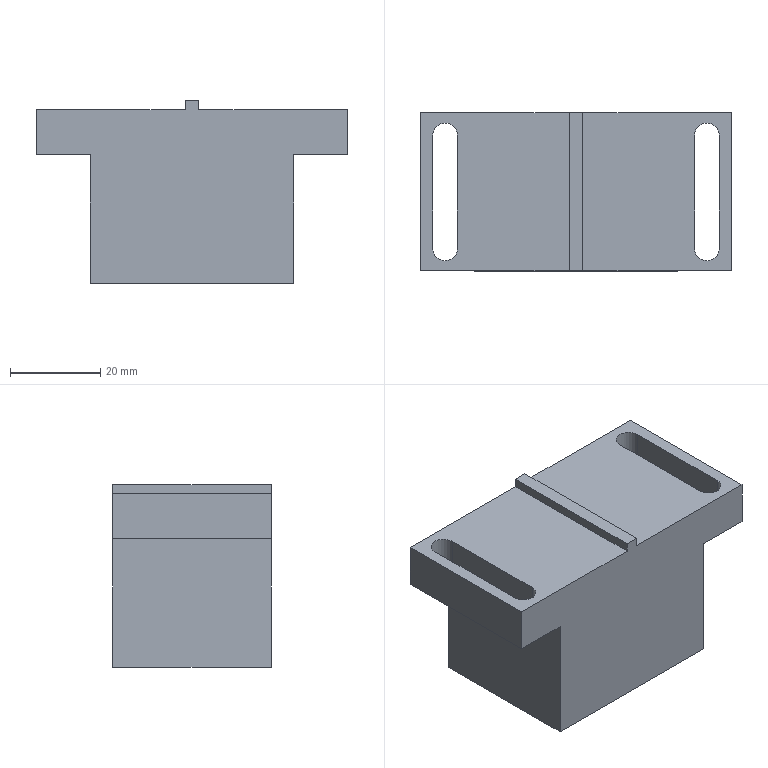Part | STEP file | 11-FG-S02811 | 1 solid | 38 faces | box 69 x 35 x 40.5 mm | volume 65665 mm3 | plane 18 | cylinder 12 | cone 8 | commonest cylinder face diameters 3.3 x8 5.5 x4
STEP:
#1=CARTESIAN_POINT('',(44.15,-7.,10.1));
#2=VERTEX_POINT('',#1);
#3=CARTESIAN_POINT('',(40.85,-7.,10.1));
#4=VERTEX_POINT('',#3);
#5=CARTESIAN_POINT('',(42.5,-7.,10.1));
#6=DIRECTION('',(0.,0.,-1.));
#7=DIRECTION('',(-1.,0.,0.));
#8=AXIS2_PLACEMENT_3D('',#5,#6,#7);
#9=CIRCLE('',#8,1.65);
#10=EDGE_CURVE('',#2,#4,#9,.T.);
#11=ORIENTED_EDGE('',*,*,#10,.F.);
#12=CARTESIAN_POINT('',(44.15,-7.,0.));
#13=VERTEX_POINT('',#12);
#14=CARTESIAN_POINT('',(44.15,-7.,0.));
#15=DIRECTION('',(0.,0.,-1.));
#16=VECTOR('',#15,1000.);
#17=LINE('',#14,#16);
#18=EDGE_CURVE('',#2,#13,#17,.T.);
#19=ORIENTED_EDGE('',*,*,#18,.T.);
#20=CARTESIAN_POINT('',(40.85,-7.,0.));
#21=VERTEX_POINT('',#20);
#22=CARTESIAN_POINT('',(42.5,-7.,0.));
#23=DIRECTION('',(0.,0.,-1.));
#24=DIRECTION('',(-1.,0.,0.));
#25=AXIS2_PLACEMENT_3D('',#22,#23,#24);
#26=CIRCLE('',#25,1.65);
#27=EDGE_CURVE('',#13,#21,#26,.T.);
#28=ORIENTED_EDGE('',*,*,#27,.T.);
#29=CARTESIAN_POINT('',(40.85,-7.,0.));
#30=DIRECTION('',(0.,0.,-1.));
#31=VECTOR('',#30,1000.);
#32=LINE('',#29,#31);
#33=EDGE_CURVE('',#4,#21,#32,.T.);
#34=ORIENTED_EDGE('',*,*,#33,.F.);
#35=EDGE_LOOP('',(#11,#19,#28,#34));
#36=FACE_OUTER_BOUND('',#35,.T.);
#37=CARTESIAN_POINT('',(42.5,-7.,0.));
#38=DIRECTION('',(0.,0.,-1.));
#39=DIRECTION('',(-1.,0.,0.));
#40=AXIS2_PLACEMENT_3D('',#37,#38,#39);
#41=CYLINDRICAL_SURFACE('',#40,1.65);
#42=ADVANCED_FACE('',(#36),#41,.F.);
#43=CARTESIAN_POINT('',(42.5,-7.,11.091));
#44=VERTEX_POINT('',#43);
#45=CARTESIAN_POINT('',(40.85,-7.,10.1));
#46=DIRECTION('',(-0.8572,0.,-0.515));
#47=VECTOR('',#46,1000.);
#48=LINE('',#45,#47);
#49=EDGE_CURVE('',#44,#4,#48,.T.);
#50=ORIENTED_EDGE('',*,*,#49,.F.);
#51=CARTESIAN_POINT('',(44.15,-7.,10.1));
#52=DIRECTION('',(0.8572,0.,-0.515));
#53=VECTOR('',#52,1000.);
#54=LINE('',#51,#53);
#55=EDGE_CURVE('',#44,#2,#54,.T.);
#56=ORIENTED_EDGE('',*,*,#55,.T.);
#57=ORIENTED_EDGE('',*,*,#10,.T.);
#58=EDGE_LOOP('',(#50,#56,#57));
#59=FACE_OUTER_BOUND('',#58,.T.);
#60=CARTESIAN_POINT('',(42.5,-7.,10.1));
#61=DIRECTION('',(0.,0.,-1.));
#62=DIRECTION('',(-1.,0.,0.));
#63=AXIS2_PLACEMENT_3D('',#60,#61,#62);
#64=CONICAL_SURFACE('',#63,1.65,1.03);
#65=ADVANCED_FACE('',(#59),#64,.F.);
#66=CARTESIAN_POINT('',(44.15,-28.,10.1));
#67=VERTEX_POINT('',#66);
#68=CARTESIAN_POINT('',(40.85,-28.,10.1));
#69=VERTEX_POINT('',#68);
#70=CARTESIAN_POINT('',(42.5,-28.,10.1));
#71=DIRECTION('',(0.,0.,-1.));
#72=DIRECTION('',(-1.,0.,0.));
#73=AXIS2_PLACEMENT_3D('',#70,#71,#72);
#74=CIRCLE('',#73,1.65);
#75=EDGE_CURVE('',#67,#69,#74,.T.);
#76=ORIENTED_EDGE('',*,*,#75,.F.);
#77=CARTESIAN_POINT('',(44.15,-28.,0.));
#78=VERTEX_POINT('',#77);
#79=CARTESIAN_POINT('',(44.15,-28.,0.));
#80=DIRECTION('',(0.,0.,-1.));
#81=VECTOR('',#80,1000.);
#82=LINE('',#79,#81);
#83=EDGE_CURVE('',#67,#78,#82,.T.);
#84=ORIENTED_EDGE('',*,*,#83,.T.);
#85=CARTESIAN_POINT('',(40.85,-28.,0.));
#86=VERTEX_POINT('',#85);
#87=CARTESIAN_POINT('',(42.5,-28.,0.));
#88=DIRECTION('',(0.,0.,-1.));
#89=DIRECTION('',(-1.,0.,0.));
#90=AXIS2_PLACEMENT_3D('',#87,#88,#89);
#91=CIRCLE('',#90,1.65);
#92=EDGE_CURVE('',#78,#86,#91,.T.);
#93=ORIENTED_EDGE('',*,*,#92,.T.);
#94=CARTESIAN_POINT('',(40.85,-28.,0.));
#95=DIRECTION('',(0.,0.,-1.));
#96=VECTOR('',#95,1000.);
#97=LINE('',#94,#96);
#98=EDGE_CURVE('',#69,#86,#97,.T.);
#99=ORIENTED_EDGE('',*,*,#98,.F.);
#100=EDGE_LOOP('',(#76,#84,#93,#99));
#101=FACE_OUTER_BOUND('',#100,.T.);
#102=CARTESIAN_POINT('',(42.5,-28.,0.));
#103=DIRECTION('',(0.,0.,-1.));
#104=DIRECTION('',(-1.,0.,0.));
#105=AXIS2_PLACEMENT_3D('',#102,#103,#104);
#106=CYLINDRICAL_SURFACE('',#105,1.65);
#107=ADVANCED_FACE('',(#101),#106,.F.);
#108=CARTESIAN_POINT('',(42.5,-28.,11.091));
#109=VERTEX_POINT('',#108);
#110=CARTESIAN_POINT('',(40.85,-28.,10.1));
#111=DIRECTION('',(-0.8572,0.,-0.515));
#112=VECTOR('',#111,1000.);
#113=LINE('',#110,#112);
#114=EDGE_CURVE('',#109,#69,#113,.T.);
#115=ORIENTED_EDGE('',*,*,#114,.F.);
#116=CARTESIAN_POINT('',(44.15,-28.,10.1));
#117=DIRECTION('',(0.8572,0.,-0.515));
#118=VECTOR('',#117,1000.);
#119=LINE('',#116,#118);
#120=EDGE_CURVE('',#109,#67,#119,.T.);
#121=ORIENTED_EDGE('',*,*,#120,.T.);
#122=ORIENTED_EDGE('',*,*,#75,.T.);
#123=EDGE_LOOP('',(#115,#121,#122));
#124=FACE_OUTER_BOUND('',#123,.T.);
#125=CARTESIAN_POINT('',(42.5,-28.,10.1));
#126=DIRECTION('',(0.,0.,-1.));
#127=DIRECTION('',(-1.,0.,0.));
#128=AXIS2_PLACEMENT_3D('',#125,#126,#127);
#129=CONICAL_SURFACE('',#128,1.65,1.03);
#130=ADVANCED_FACE('',(#124),#129,.F.);
#131=CARTESIAN_POINT('',(6.15,-28.,10.1));
#132=VERTEX_POINT('',#131);
#133=CARTESIAN_POINT('',(2.85,-28.,10.1));
#134=VERTEX_POINT('',#133);
#135=CARTESIAN_POINT('',(4.5,-28.,10.1));
#136=DIRECTION('',(0.,0.,-1.));
#137=DIRECTION('',(-1.,0.,0.));
#138=AXIS2_PLACEMENT_3D('',#135,#136,#137);
#139=CIRCLE('',#138,1.65);
#140=EDGE_CURVE('',#132,#134,#139,.T.);
#141=ORIENTED_EDGE('',*,*,#140,.F.);
#142=CARTESIAN_POINT('',(6.15,-28.,0.));
#143=VERTEX_POINT('',#142);
#144=CARTESIAN_POINT('',(6.15,-28.,0.));
#145=DIRECTION('',(0.,0.,-1.));
#146=VECTOR('',#145,1000.);
#147=LINE('',#144,#146);
#148=EDGE_CURVE('',#132,#143,#147,.T.);
#149=ORIENTED_EDGE('',*,*,#148,.T.);
#150=CARTESIAN_POINT('',(2.85,-28.,0.));
#151=VERTEX_POINT('',#150);
#152=CARTESIAN_POINT('',(4.5,-28.,0.));
#153=DIRECTION('',(0.,0.,-1.));
#154=DIRECTION('',(-1.,0.,0.));
#155=AXIS2_PLACEMENT_3D('',#152,#153,#154);
#156=CIRCLE('',#155,1.65);
#157=EDGE_CURVE('',#143,#151,#156,.T.);
#158=ORIENTED_EDGE('',*,*,#157,.T.);
#159=CARTESIAN_POINT('',(2.85,-28.,0.));
#160=DIRECTION('',(0.,0.,-1.));
#161=VECTOR('',#160,1000.);
#162=LINE('',#159,#161);
#163=EDGE_CURVE('',#134,#151,#162,.T.);
#164=ORIENTED_EDGE('',*,*,#163,.F.);
#165=EDGE_LOOP('',(#141,#149,#158,#164));
#166=FACE_OUTER_BOUND('',#165,.T.);
#167=CARTESIAN_POINT('',(4.5,-28.,0.));
#168=DIRECTION('',(0.,0.,-1.));
#169=DIRECTION('',(-1.,0.,0.));
#170=AXIS2_PLACEMENT_3D('',#167,#168,#169);
#171=CYLINDRICAL_SURFACE('',#170,1.65);
#172=ADVANCED_FACE('',(#166),#171,.F.);
#173=CARTESIAN_POINT('',(4.5,-28.,11.091));
#174=VERTEX_POINT('',#173);
#175=CARTESIAN_POINT('',(2.85,-28.,10.1));
#176=DIRECTION('',(-0.8572,0.,-0.515));
#177=VECTOR('',#176,1000.);
#178=LINE('',#175,#177);
#179=EDGE_CURVE('',#174,#134,#178,.T.);
#180=ORIENTED_EDGE('',*,*,#179,.F.);
#181=CARTESIAN_POINT('',(6.15,-28.,10.1));
#182=DIRECTION('',(0.8572,0.,-0.515));
#183=VECTOR('',#182,1000.);
#184=LINE('',#181,#183);
#185=EDGE_CURVE('',#174,#132,#184,.T.);
#186=ORIENTED_EDGE('',*,*,#185,.T.);
#187=ORIENTED_EDGE('',*,*,#140,.T.);
#188=EDGE_LOOP('',(#180,#186,#187));
#189=FACE_OUTER_BOUND('',#188,.T.);
#190=CARTESIAN_POINT('',(4.5,-28.,10.1));
#191=DIRECTION('',(0.,0.,-1.));
#192=DIRECTION('',(-1.,0.,0.));
#193=AXIS2_PLACEMENT_3D('',#190,#191,#192);
#194=CONICAL_SURFACE('',#193,1.65,1.03);
#195=ADVANCED_FACE('',(#189),#194,.F.);
#196=CARTESIAN_POINT('',(6.15,-7.,10.1));
#197=VERTEX_POINT('',#196);
#198=CARTESIAN_POINT('',(2.85,-7.,10.1));
#199=VERTEX_POINT('',#198);
#200=CARTESIAN_POINT('',(4.5,-7.,10.1));
#201=DIRECTION('',(0.,0.,-1.));
#202=DIRECTION('',(-1.,0.,0.));
#203=AXIS2_PLACEMENT_3D('',#200,#201,#202);
#204=CIRCLE('',#203,1.65);
#205=EDGE_CURVE('',#197,#199,#204,.T.);
#206=ORIENTED_EDGE('',*,*,#205,.F.);
#207=CARTESIAN_POINT('',(6.15,-7.,0.));
#208=VERTEX_POINT('',#207);
#209=CARTESIAN_POINT('',(6.15,-7.,0.));
#210=DIRECTION('',(0.,0.,-1.));
#211=VECTOR('',#210,1000.);
#212=LINE('',#209,#211);
#213=EDGE_CURVE('',#197,#208,#212,.T.);
#214=ORIENTED_EDGE('',*,*,#213,.T.);
#215=CARTESIAN_POINT('',(2.85,-7.,0.));
#216=VERTEX_POINT('',#215);
#217=CARTESIAN_POINT('',(4.5,-7.,0.));
#218=DIRECTION('',(0.,0.,-1.));
#219=DIRECTION('',(-1.,0.,0.));
#220=AXIS2_PLACEMENT_3D('',#217,#218,#219);
#221=CIRCLE('',#220,1.65);
#222=EDGE_CURVE('',#208,#216,#221,.T.);
#223=ORIENTED_EDGE('',*,*,#222,.T.);
#224=CARTESIAN_POINT('',(2.85,-7.,0.));
#225=DIRECTION('',(0.,0.,-1.));
#226=VECTOR('',#225,1000.);
#227=LINE('',#224,#226);
#228=EDGE_CURVE('',#199,#216,#227,.T.);
#229=ORIENTED_EDGE('',*,*,#228,.F.);
#230=EDGE_LOOP('',(#206,#214,#223,#229));
#231=FACE_OUTER_BOUND('',#230,.T.);
#232=CARTESIAN_POINT('',(4.5,-7.,0.));
#233=DIRECTION('',(0.,0.,-1.));
#234=DIRECTION('',(-1.,0.,0.));
#235=AXIS2_PLACEMENT_3D('',#232,#233,#234);
#236=CYLINDRICAL_SURFACE('',#235,1.65);
#237=ADVANCED_FACE('',(#231),#236,.F.);
#238=CARTESIAN_POINT('',(4.5,-7.,11.091));
#239=VERTEX_POINT('',#238);
#240=CARTESIAN_POINT('',(2.85,-7.,10.1));
#241=DIRECTION('',(-0.8572,0.,-0.515));
#242=VECTOR('',#241,1000.);
#243=LINE('',#240,#242);
#244=EDGE_CURVE('',#239,#199,#243,.T.);
#245=ORIENTED_EDGE('',*,*,#244,.F.);
#246=CARTESIAN_POINT('',(6.15,-7.,10.1));
#247=DIRECTION('',(0.8572,0.,-0.515));
#248=VECTOR('',#247,1000.);
#249=LINE('',#246,#248);
#250=EDGE_CURVE('',#239,#197,#249,.T.);
#251=ORIENTED_EDGE('',*,*,#250,.T.);
#252=ORIENTED_EDGE('',*,*,#205,.T.);
#253=EDGE_LOOP('',(#245,#251,#252));
#254=FACE_OUTER_BOUND('',#253,.T.);
#255=CARTESIAN_POINT('',(4.5,-7.,10.1));
#256=DIRECTION('',(0.,0.,-1.));
#257=DIRECTION('',(-1.,0.,0.));
#258=AXIS2_PLACEMENT_3D('',#255,#256,#257);
#259=CONICAL_SURFACE('',#258,1.65,1.03);
#260=ADVANCED_FACE('',(#254),#259,.F.);
#261=CARTESIAN_POINT('',(55.25,-5.,38.5));
#262=VERTEX_POINT('',#261);
#263=CARTESIAN_POINT('',(49.75,-5.,38.5));
#264=VERTEX_POINT('',#263);
#265=CARTESIAN_POINT('',(52.5,-5.,38.5));
#266=DIRECTION('',(0.,0.,1.));
#267=DIRECTION('',(1.,0.,0.));
#268=AXIS2_PLACEMENT_3D('',#265,#266,#267);
#269=CIRCLE('',#268,2.75);
#270=EDGE_CURVE('',#262,#264,#269,.T.);
#271=ORIENTED_EDGE('',*,*,#270,.F.);
#272=CARTESIAN_POINT('',(55.25,-30.,38.5));
#273=VERTEX_POINT('',#272);
#274=CARTESIAN_POINT('',(55.25,0.,38.5));
#275=DIRECTION('',(0.,1.,0.));
#276=VECTOR('',#275,1000.);
#277=LINE('',#274,#276);
#278=EDGE_CURVE('',#273,#262,#277,.T.);
#279=ORIENTED_EDGE('',*,*,#278,.F.);
#280=CARTESIAN_POINT('',(49.75,-30.,38.5));
#281=VERTEX_POINT('',#280);
#282=CARTESIAN_POINT('',(52.5,-30.,38.5));
#283=DIRECTION('',(0.,0.,1.));
#284=DIRECTION('',(1.,0.,0.));
#285=AXIS2_PLACEMENT_3D('',#282,#283,#284);
#286=CIRCLE('',#285,2.75);
#287=EDGE_CURVE('',#281,#273,#286,.T.);
#288=ORIENTED_EDGE('',*,*,#287,.F.);
#289=CARTESIAN_POINT('',(49.75,0.,38.5));
#290=DIRECTION('',(0.,-1.,0.));
#291=VECTOR('',#290,1000.);
#292=LINE('',#289,#291);
#293=EDGE_CURVE('',#264,#281,#292,.T.);
#294=ORIENTED_EDGE('',*,*,#293,.F.);
#295=EDGE_LOOP('',(#271,#279,#288,#294));
#296=FACE_BOUND('',#295,.T.);
#297=CARTESIAN_POINT('',(58.,0.,38.5));
#298=VERTEX_POINT('',#297);
#299=CARTESIAN_POINT('',(25.,0.,38.5));
#300=VERTEX_POINT('',#299);
#301=CARTESIAN_POINT('',(0.,0.,38.5));
#302=DIRECTION('',(-1.,0.,0.));
#303=VECTOR('',#302,1000.);
#304=LINE('',#301,#303);
#305=EDGE_CURVE('',#298,#300,#304,.T.);
#306=ORIENTED_EDGE('',*,*,#305,.T.);
#307=CARTESIAN_POINT('',(25.,-35.,38.5));
#308=VERTEX_POINT('',#307);
#309=CARTESIAN_POINT('',(25.,3.606,38.5));
#310=DIRECTION('',(0.,-1.,0.));
#311=VECTOR('',#310,1000.);
#312=LINE('',#309,#311);
#313=EDGE_CURVE('',#300,#308,#312,.T.);
#314=ORIENTED_EDGE('',*,*,#313,.T.);
#315=CARTESIAN_POINT('',(58.,-35.,38.5));
#316=VERTEX_POINT('',#315);
#317=CARTESIAN_POINT('',(0.,-35.,38.5));
#318=DIRECTION('',(1.,0.,0.));
#319=VECTOR('',#318,1000.);
#320=LINE('',#317,#319);
#321=EDGE_CURVE('',#308,#316,#320,.T.);
#322=ORIENTED_EDGE('',*,*,#321,.T.);
#323=CARTESIAN_POINT('',(58.,0.,38.5));
#324=DIRECTION('',(0.,1.,0.));
#325=VECTOR('',#324,1000.);
#326=LINE('',#323,#325);
#327=EDGE_CURVE('',#316,#298,#326,.T.);
#328=ORIENTED_EDGE('',*,*,#327,.T.);
#329=EDGE_LOOP('',(#306,#314,#322,#328));
#330=FACE_OUTER_BOUND('',#329,.T.);
#331=CARTESIAN_POINT('',(0.,0.,38.5));
#332=DIRECTION('',(0.,0.,1.));
#333=DIRECTION('',(1.,0.,0.));
#334=AXIS2_PLACEMENT_3D('',#331,#332,#333);
#335=PLANE('',#334);
#336=ADVANCED_FACE('',(#296,#330),#335,.T.);
#337=CARTESIAN_POINT('',(-11.,-35.,38.5));
#338=VERTEX_POINT('',#337);
#339=CARTESIAN_POINT('',(22.,-35.,38.5));
#340=VERTEX_POINT('',#339);
#341=CARTESIAN_POINT('',(0.,-35.,38.5));
#342=DIRECTION('',(1.,0.,0.));
#343=VECTOR('',#342,1000.);
#344=LINE('',#341,#343);
#345=EDGE_CURVE('',#338,#340,#344,.T.);
#346=ORIENTED_EDGE('',*,*,#345,.F.);
#347=CARTESIAN_POINT('',(-11.,-35.,28.5));
#348=VERTEX_POINT('',#347);
#349=CARTESIAN_POINT('',(-11.,-35.,28.5));
#350=DIRECTION('',(0.,0.,1.));
#351=VECTOR('',#350,1000.);
#352=LINE('',#349,#351);
#353=EDGE_CURVE('',#348,#338,#352,.T.);
#354=ORIENTED_EDGE('',*,*,#353,.F.);
#355=CARTESIAN_POINT('',(1.,-35.,28.5));
#356=VERTEX_POINT('',#355);
#357=CARTESIAN_POINT('',(1.,-35.,28.5));
#358=DIRECTION('',(1.,0.,0.));
#359=VECTOR('',#358,1000.);
#360=LINE('',#357,#359);
#361=EDGE_CURVE('',#348,#356,#360,.T.);
#362=ORIENTED_EDGE('',*,*,#361,.T.);
#363=CARTESIAN_POINT('',(1.,-35.,0.));
#364=VERTEX_POINT('',#363);
#365=CARTESIAN_POINT('',(1.,-35.,38.5));
#366=DIRECTION('',(0.,0.,-1.));
#367=VECTOR('',#366,1000.);
#368=LINE('',#365,#367);
#369=EDGE_CURVE('',#356,#364,#368,.T.);
#370=ORIENTED_EDGE('',*,*,#369,.T.);
#371=CARTESIAN_POINT('',(46.,-35.,0.));
#372=VERTEX_POINT('',#371);
#373=CARTESIAN_POINT('',(0.,-35.,0.));
#374=DIRECTION('',(1.,0.,0.));
#375=VECTOR('',#374,1000.);
#376=LINE('',#373,#375);
#377=EDGE_CURVE('',#364,#372,#376,.T.);
#378=ORIENTED_EDGE('',*,*,#377,.T.);
#379=CARTESIAN_POINT('',(46.,-35.,28.5));
#380=VERTEX_POINT('',#379);
#381=CARTESIAN_POINT('',(46.,-35.,38.5));
#382=DIRECTION('',(0.,0.,-1.));
#383=VECTOR('',#382,1000.);
#384=LINE('',#381,#383);
#385=EDGE_CURVE('',#380,#372,#384,.T.);
#386=ORIENTED_EDGE('',*,*,#385,.F.);
#387=CARTESIAN_POINT('',(58.,-35.,28.5));
#388=VERTEX_POINT('',#387);
#389=CARTESIAN_POINT('',(46.,-35.,28.5));
#390=DIRECTION('',(1.,0.,0.));
#391=VECTOR('',#390,1000.);
#392=LINE('',#389,#391);
#393=EDGE_CURVE('',#380,#388,#392,.T.);
#394=ORIENTED_EDGE('',*,*,#393,.T.);
#395=CARTESIAN_POINT('',(58.,-35.,28.5));
#396=DIRECTION('',(0.,0.,1.));
#397=VECTOR('',#396,1000.);
#398=LINE('',#395,#397);
#399=EDGE_CURVE('',#388,#316,#398,.T.);
#400=ORIENTED_EDGE('',*,*,#399,.T.);
#401=ORIENTED_EDGE('',*,*,#321,.F.);
#402=CARTESIAN_POINT('',(25.,-35.,40.5));
#403=VERTEX_POINT('',#402);
#404=CARTESIAN_POINT('',(25.,-35.,40.5));
#405=DIRECTION('',(0.,0.,1.));
#406=VECTOR('',#405,1000.);
#407=LINE('',#404,#406);
#408=EDGE_CURVE('',#308,#403,#407,.T.);
#409=ORIENTED_EDGE('',*,*,#408,.T.);
#410=CARTESIAN_POINT('',(22.,-35.,40.5));
#411=VERTEX_POINT('',#410);
#412=CARTESIAN_POINT('',(25.,-35.,40.5));
#413=DIRECTION('',(-1.,0.,0.));
#414=VECTOR('',#413,1000.);
#415=LINE('',#412,#414);
#416=EDGE_CURVE('',#403,#411,#415,.T.);
#417=ORIENTED_EDGE('',*,*,#416,.T.);
#418=CARTESIAN_POINT('',(22.,-35.,40.5));
#419=DIRECTION('',(0.,0.,-1.));
#420=VECTOR('',#419,1000.);
#421=LINE('',#418,#420);
#422=EDGE_CURVE('',#411,#340,#421,.T.);
#423=ORIENTED_EDGE('',*,*,#422,.T.);
#424=EDGE_LOOP('',(#346,#354,#362,#370,#378,#386,#394,#400,#401,#409,#417,#423));
#425=FACE_OUTER_BOUND('',#424,.T.);
#426=CARTESIAN_POINT('',(0.,-35.,38.5));
#427=DIRECTION('',(0.,1.,0.));
#428=DIRECTION('',(0.,0.,1.));
#429=AXIS2_PLACEMENT_3D('',#426,#427,#428);
#430=PLANE('',#429);
#431=ADVANCED_FACE('',(#425),#430,.F.);
#432=CARTESIAN_POINT('',(46.,0.,28.5));
#433=VERTEX_POINT('',#432);
#434=CARTESIAN_POINT('',(46.,0.,0.));
#435=VERTEX_POINT('',#434);
#436=CARTESIAN_POINT('',(46.,0.,38.5));
#437=DIRECTION('',(0.,0.,-1.));
#438=VECTOR('',#437,1000.);
#439=LINE('',#436,#438);
#440=EDGE_CURVE('',#433,#435,#439,.T.);
#441=ORIENTED_EDGE('',*,*,#440,.F.);
#442=CARTESIAN_POINT('',(46.,0.,28.5));
#443=DIRECTION('',(0.,-1.,0.));
#444=VECTOR('',#443,1000.);
#445=LINE('',#442,#444);
#446=EDGE_CURVE('',#433,#380,#445,.T.);
#447=ORIENTED_EDGE('',*,*,#446,.T.);
#448=ORIENTED_EDGE('',*,*,#385,.T.);
#449=CARTESIAN_POINT('',(46.,0.,0.));
#450=DIRECTION('',(0.,1.,0.));
#451=VECTOR('',#450,1000.);
#452=LINE('',#449,#451);
#453=EDGE_CURVE('',#372,#435,#452,.T.);
#454=ORIENTED_EDGE('',*,*,#453,.T.);
#455=EDGE_LOOP('',(#441,#447,#448,#454));
#456=FACE_OUTER_BOUND('',#455,.T.);
#457=CARTESIAN_POINT('',(46.,0.,38.5));
#458=DIRECTION('',(-1.,0.,0.));
#459=DIRECTION('',(0.,0.,1.));
#460=AXIS2_PLACEMENT_3D('',#457,#458,#459);
#461=PLANE('',#460);
#462=ADVANCED_FACE('',(#456),#461,.F.);
#463=CARTESIAN_POINT('',(1.,0.,0.));
#464=VERTEX_POINT('',#463);
#465=CARTESIAN_POINT('',(0.,0.,0.));
#466=DIRECTION('',(-1.,0.,0.));
#467=VECTOR('',#466,1000.);
#468=LINE('',#465,#467);
#469=EDGE_CURVE('',#435,#464,#468,.T.);
#470=ORIENTED_EDGE('',*,*,#469,.T.);
#471=CARTESIAN_POINT('',(1.,0.,28.5));
#472=VERTEX_POINT('',#471);
#473=CARTESIAN_POINT('',(1.,0.,0.));
#474=DIRECTION('',(0.,0.,-1.));
#475=VECTOR('',#474,1000.);
#476=LINE('',#473,#475);
#477=EDGE_CURVE('',#472,#464,#476,.T.);
#478=ORIENTED_EDGE('',*,*,#477,.F.);
#479=CARTESIAN_POINT('',(-11.,0.,28.5));
#480=VERTEX_POINT('',#479);
#481=CARTESIAN_POINT('',(1.,0.,28.5));
#482=DIRECTION('',(-1.,0.,0.));
#483=VECTOR('',#482,1000.);
#484=LINE('',#481,#483);
#485=EDGE_CURVE('',#472,#480,#484,.T.);
#486=ORIENTED_EDGE('',*,*,#485,.T.);
#487=CARTESIAN_POINT('',(-11.,0.,38.5));
#488=VERTEX_POINT('',#487);
#489=CARTESIAN_POINT('',(-11.,0.,28.5));
#490=DIRECTION('',(0.,0.,1.));
#491=VECTOR('',#490,1000.);
#492=LINE('',#489,#491);
#493=EDGE_CURVE('',#480,#488,#492,.T.);
#494=ORIENTED_EDGE('',*,*,#493,.T.);
#495=CARTESIAN_POINT('',(22.,0.,38.5));
#496=VERTEX_POINT('',#495);
#497=CARTESIAN_POINT('',(0.,0.,38.5));
#498=DIRECTION('',(-1.,0.,0.));
#499=VECTOR('',#498,1000.);
#500=LINE('',#497,#499);
#501=EDGE_CURVE('',#496,#488,#500,.T.);
#502=ORIENTED_EDGE('',*,*,#501,.F.);
#503=CARTESIAN_POINT('',(22.,0.,40.5));
#504=VERTEX_POINT('',#503);
#505=CARTESIAN_POINT('',(22.,0.,40.5));
#506=DIRECTION('',(0.,0.,1.));
#507=VECTOR('',#506,1000.);
#508=LINE('',#505,#507);
#509=EDGE_CURVE('',#496,#504,#508,.T.);
#510=ORIENTED_EDGE('',*,*,#509,.T.);
#511=CARTESIAN_POINT('',(25.,0.,40.5));
#512=VERTEX_POINT('',#511);
#513=CARTESIAN_POINT('',(25.,0.,40.5));
#514=DIRECTION('',(1.,0.,0.));
#515=VECTOR('',#514,1000.);
#516=LINE('',#513,#515);
#517=EDGE_CURVE('',#504,#512,#516,.T.);
#518=ORIENTED_EDGE('',*,*,#517,.T.);
#519=CARTESIAN_POINT('',(25.,0.,40.5));
#520=DIRECTION('',(0.,0.,-1.));
#521=VECTOR('',#520,1000.);
#522=LINE('',#519,#521);
#523=EDGE_CURVE('',#512,#300,#522,.T.);
#524=ORIENTED_EDGE('',*,*,#523,.T.);
#525=ORIENTED_EDGE('',*,*,#305,.F.);
#526=CARTESIAN_POINT('',(58.,0.,28.5));
#527=VERTEX_POINT('',#526);
#528=CARTESIAN_POINT('',(58.,0.,28.5));
#529=DIRECTION('',(0.,0.,1.));
#530=VECTOR('',#529,1000.);
#531=LINE('',#528,#530);
#532=EDGE_CURVE('',#527,#298,#531,.T.);
#533=ORIENTED_EDGE('',*,*,#532,.F.);
#534=CARTESIAN_POINT('',(46.,0.,28.5));
#535=DIRECTION('',(-1.,0.,0.));
#536=VECTOR('',#535,1000.);
#537=LINE('',#534,#536);
#538=EDGE_CURVE('',#527,#433,#537,.T.);
#539=ORIENTED_EDGE('',*,*,#538,.T.);
#540=ORIENTED_EDGE('',*,*,#440,.T.);
#541=EDGE_LOOP('',(#470,#478,#486,#494,#502,#510,#518,#524,#525,#533,#539,#540));
#542=FACE_OUTER_BOUND('',#541,.T.);
#543=CARTESIAN_POINT('',(0.,0.,38.5));
#544=DIRECTION('',(0.,-1.,0.));
#545=DIRECTION('',(0.,0.,-1.));
#546=AXIS2_PLACEMENT_3D('',#543,#544,#545);
#547=PLANE('',#546);
#548=ADVANCED_FACE('',(#542),#547,.F.);
#549=CARTESIAN_POINT('',(22.,3.606,38.5));
#550=DIRECTION('',(0.,-1.,0.));
#551=VECTOR('',#550,1000.);
#552=LINE('',#549,#551);
#553=EDGE_CURVE('',#496,#340,#552,.T.);
#554=ORIENTED_EDGE('',*,*,#553,.F.);
#555=ORIENTED_EDGE('',*,*,#501,.T.);
#556=CARTESIAN_POINT('',(-11.,0.,38.5));
#557=DIRECTION('',(0.,-1.,0.));
#558=VECTOR('',#557,1000.);
#559=LINE('',#556,#558);
#560=EDGE_CURVE('',#488,#338,#559,.T.);
#561=ORIENTED_EDGE('',*,*,#560,.T.);
#562=ORIENTED_EDGE('',*,*,#345,.T.);
#563=EDGE_LOOP('',(#554,#555,#561,#562));
#564=FACE_OUTER_BOUND('',#563,.T.);
#565=CARTESIAN_POINT('',(-2.75,-5.,38.5));
#566=VERTEX_POINT('',#565);
#567=CARTESIAN_POINT('',(-8.25,-5.,38.5));
#568=VERTEX_POINT('',#567);
#569=CARTESIAN_POINT('',(-5.5,-5.,38.5));
#570=DIRECTION('',(0.,0.,1.));
#571=DIRECTION('',(1.,0.,0.));
#572=AXIS2_PLACEMENT_3D('',#569,#570,#571);
#573=CIRCLE('',#572,2.75);
#574=EDGE_CURVE('',#566,#568,#573,.T.);
#575=ORIENTED_EDGE('',*,*,#574,.F.);
#576=CARTESIAN_POINT('',(-2.75,-30.,38.5));
#577=VERTEX_POINT('',#576);
#578=CARTESIAN_POINT('',(-2.75,0.,38.5));
#579=DIRECTION('',(0.,1.,0.));
#580=VECTOR('',#579,1000.);
#581=LINE('',#578,#580);
#582=EDGE_CURVE('',#577,#566,#581,.T.);
#583=ORIENTED_EDGE('',*,*,#582,.F.);
#584=CARTESIAN_POINT('',(-8.25,-30.,38.5));
#585=VERTEX_POINT('',#584);
#586=CARTESIAN_POINT('',(-5.5,-30.,38.5));
#587=DIRECTION('',(0.,0.,1.));
#588=DIRECTION('',(1.,0.,0.));
#589=AXIS2_PLACEMENT_3D('',#586,#587,#588);
#590=CIRCLE('',#589,2.75);
#591=EDGE_CURVE('',#585,#577,#590,.T.);
#592=ORIENTED_EDGE('',*,*,#591,.F.);
#593=CARTESIAN_POINT('',(-8.25,0.,38.5));
#594=DIRECTION('',(0.,-1.,0.));
#595=VECTOR('',#594,1000.);
#596=LINE('',#593,#595);
#597=EDGE_CURVE('',#568,#585,#596,.T.);
#598=ORIENTED_EDGE('',*,*,#597,.F.);
#599=EDGE_LOOP('',(#575,#583,#592,#598));
#600=FACE_BOUND('',#599,.T.);
#601=CARTESIAN_POINT('',(0.,0.,38.5));
#602=DIRECTION('',(0.,0.,1.));
#603=DIRECTION('',(1.,0.,0.));
#604=AXIS2_PLACEMENT_3D('',#601,#602,#603);
#605=PLANE('',#604);
#606=ADVANCED_FACE('',(#564,#600),#605,.T.);
#607=CARTESIAN_POINT('',(42.5,-7.,0.));
#608=DIRECTION('',(0.,0.,-1.));
#609=DIRECTION('',(-1.,0.,0.));
#610=AXIS2_PLACEMENT_3D('',#607,#608,#609);
#611=CIRCLE('',#610,1.65);
#612=EDGE_CURVE('',#21,#13,#611,.T.);
#613=ORIENTED_EDGE('',*,*,#612,.F.);
#614=ORIENTED_EDGE('',*,*,#27,.F.);
#615=EDGE_LOOP('',(#613,#614));
#616=FACE_BOUND('',#615,.T.);
#617=CARTESIAN_POINT('',(42.5,-28.,0.));
#618=DIRECTION('',(0.,0.,-1.));
#619=DIRECTION('',(-1.,0.,0.));
#620=AXIS2_PLACEMENT_3D('',#617,#618,#619);
#621=CIRCLE('',#620,1.65);
#622=EDGE_CURVE('',#86,#78,#621,.T.);
#623=ORIENTED_EDGE('',*,*,#622,.F.);
#624=ORIENTED_EDGE('',*,*,#92,.F.);
#625=EDGE_LOOP('',(#623,#624));
#626=FACE_BOUND('',#625,.T.);
#627=CARTESIAN_POINT('',(4.5,-28.,0.));
#628=DIRECTION('',(0.,0.,-1.));
#629=DIRECTION('',(-1.,0.,0.));
#630=AXIS2_PLACEMENT_3D('',#627,#628,#629);
#631=CIRCLE('',#630,1.65);
#632=EDGE_CURVE('',#151,#143,#631,.T.);
#633=ORIENTED_EDGE('',*,*,#632,.F.);
#634=ORIENTED_EDGE('',*,*,#157,.F.);
#635=EDGE_LOOP('',(#633,#634));
#636=FACE_BOUND('',#635,.T.);
#637=CARTESIAN_POINT('',(4.5,-7.,0.));
#638=DIRECTION('',(0.,0.,-1.));
#639=DIRECTION('',(-1.,0.,0.));
#640=AXIS2_PLACEMENT_3D('',#637,#638,#639);
#641=CIRCLE('',#640,1.65);
#642=EDGE_CURVE('',#216,#208,#641,.T.);
#643=ORIENTED_EDGE('',*,*,#642,.F.);
#644=ORIENTED_EDGE('',*,*,#222,.F.);
#645=EDGE_LOOP('',(#643,#644));
#646=FACE_BOUND('',#645,.T.);
#647=ORIENTED_EDGE('',*,*,#377,.F.);
#648=CARTESIAN_POINT('',(1.,0.,0.));
#649=DIRECTION('',(0.,1.,0.));
#650=VECTOR('',#649,1000.);
#651=LINE('',#648,#650);
#652=EDGE_CURVE('',#364,#464,#651,.T.);
#653=ORIENTED_EDGE('',*,*,#652,.T.);
#654=ORIENTED_EDGE('',*,*,#469,.F.);
#655=ORIENTED_EDGE('',*,*,#453,.F.);
#656=EDGE_LOOP('',(#647,#653,#654,#655));
#657=FACE_OUTER_BOUND('',#656,.T.);
#658=CARTESIAN_POINT('',(0.,0.,0.));
#659=DIRECTION('',(0.,0.,1.));
#660=DIRECTION('',(1.,0.,0.));
#661=AXIS2_PLACEMENT_3D('',#658,#659,#660);
#662=PLANE('',#661);
#663=ADVANCED_FACE('',(#616,#626,#636,#646,#657),#662,.F.);
#664=ORIENTED_EDGE('',*,*,#369,.F.);
#665=CARTESIAN_POINT('',(1.,0.,28.5));
#666=DIRECTION('',(0.,1.,0.));
#667=VECTOR('',#666,1000.);
#668=LINE('',#665,#667);
#669=EDGE_CURVE('',#356,#472,#668,.T.);
#670=ORIENTED_EDGE('',*,*,#669,.T.);
#671=ORIENTED_EDGE('',*,*,#477,.T.);
#672=ORIENTED_EDGE('',*,*,#652,.F.);
#673=EDGE_LOOP('',(#664,#670,#671,#672));
#674=FACE_OUTER_BOUND('',#673,.T.);
#675=CARTESIAN_POINT('',(1.,-42.,0.));
#676=DIRECTION('',(1.,0.,0.));
#677=DIRECTION('',(0.,0.,-1.));
#678=AXIS2_PLACEMENT_3D('',#675,#676,#677);
#679=PLANE('',#678);
#680=ADVANCED_FACE('',(#674),#679,.F.);
#681=ORIENTED_EDGE('',*,*,#250,.F.);
#682=ORIENTED_EDGE('',*,*,#244,.T.);
#683=CARTESIAN_POINT('',(4.5,-7.,10.1));
#684=DIRECTION('',(0.,0.,-1.));
#685=DIRECTION('',(-1.,0.,0.));
#686=AXIS2_PLACEMENT_3D('',#683,#684,#685);
#687=CIRCLE('',#686,1.65);
#688=EDGE_CURVE('',#199,#197,#687,.T.);
#689=ORIENTED_EDGE('',*,*,#688,.T.);
#690=EDGE_LOOP('',(#681,#682,#689));
#691=FACE_OUTER_BOUND('',#690,.T.);
#692=CARTESIAN_POINT('',(4.5,-7.,10.1));
#693=DIRECTION('',(0.,0.,-1.));
#694=DIRECTION('',(-1.,0.,0.));
#695=AXIS2_PLACEMENT_3D('',#692,#693,#694);
#696=CONICAL_SURFACE('',#695,1.65,1.03);
#697=ADVANCED_FACE('',(#691),#696,.F.);
#698=ORIENTED_EDGE('',*,*,#213,.F.);
#699=ORIENTED_EDGE('',*,*,#688,.F.);
#700=ORIENTED_EDGE('',*,*,#228,.T.);
#701=ORIENTED_EDGE('',*,*,#642,.T.);
#702=EDGE_LOOP('',(#698,#699,#700,#701));
#703=FACE_OUTER_BOUND('',#702,.T.);
#704=CARTESIAN_POINT('',(4.5,-7.,0.));
#705=DIRECTION('',(0.,0.,-1.));
#706=DIRECTION('',(-1.,0.,0.));
#707=AXIS2_PLACEMENT_3D('',#704,#705,#706);
#708=CYLINDRICAL_SURFACE('',#707,1.65);
#709=ADVANCED_FACE('',(#703),#708,.F.);
#710=ORIENTED_EDGE('',*,*,#185,.F.);
#711=ORIENTED_EDGE('',*,*,#179,.T.);
#712=CARTESIAN_POINT('',(4.5,-28.,10.1));
#713=DIRECTION('',(0.,0.,-1.));
#714=DIRECTION('',(-1.,0.,0.));
#715=AXIS2_PLACEMENT_3D('',#712,#713,#714);
#716=CIRCLE('',#715,1.65);
#717=EDGE_CURVE('',#134,#132,#716,.T.);
#718=ORIENTED_EDGE('',*,*,#717,.T.);
#719=EDGE_LOOP('',(#710,#711,#718));
#720=FACE_OUTER_BOUND('',#719,.T.);
#721=CARTESIAN_POINT('',(4.5,-28.,10.1));
#722=DIRECTION('',(0.,0.,-1.));
#723=DIRECTION('',(-1.,0.,0.));
#724=AXIS2_PLACEMENT_3D('',#721,#722,#723);
#725=CONICAL_SURFACE('',#724,1.65,1.03);
#726=ADVANCED_FACE('',(#720),#725,.F.);
#727=ORIENTED_EDGE('',*,*,#148,.F.);
#728=ORIENTED_EDGE('',*,*,#717,.F.);
#729=ORIENTED_EDGE('',*,*,#163,.T.);
#730=ORIENTED_EDGE('',*,*,#632,.T.);
#731=EDGE_LOOP('',(#727,#728,#729,#730));
#732=FACE_OUTER_BOUND('',#731,.T.);
#733=CARTESIAN_POINT('',(4.5,-28.,0.));
#734=DIRECTION('',(0.,0.,-1.));
#735=DIRECTION('',(-1.,0.,0.));
#736=AXIS2_PLACEMENT_3D('',#733,#734,#735);
#737=CYLINDRICAL_SURFACE('',#736,1.65);
#738=ADVANCED_FACE('',(#732),#737,.F.);
#739=ORIENTED_EDGE('',*,*,#120,.F.);
#740=ORIENTED_EDGE('',*,*,#114,.T.);
#741=CARTESIAN_POINT('',(42.5,-28.,10.1));
#742=DIRECTION('',(0.,0.,-1.));
#743=DIRECTION('',(-1.,0.,0.));
#744=AXIS2_PLACEMENT_3D('',#741,#742,#743);
#745=CIRCLE('',#744,1.65);
#746=EDGE_CURVE('',#69,#67,#745,.T.);
#747=ORIENTED_EDGE('',*,*,#746,.T.);
#748=EDGE_LOOP('',(#739,#740,#747));
#749=FACE_OUTER_BOUND('',#748,.T.);
#750=CARTESIAN_POINT('',(42.5,-28.,10.1));
#751=DIRECTION('',(0.,0.,-1.));
#752=DIRECTION('',(-1.,0.,0.));
#753=AXIS2_PLACEMENT_3D('',#750,#751,#752);
#754=CONICAL_SURFACE('',#753,1.65,1.03);
#755=ADVANCED_FACE('',(#749),#754,.F.);
#756=ORIENTED_EDGE('',*,*,#83,.F.);
#757=ORIENTED_EDGE('',*,*,#746,.F.);
#758=ORIENTED_EDGE('',*,*,#98,.T.);
#759=ORIENTED_EDGE('',*,*,#622,.T.);
#760=EDGE_LOOP('',(#756,#757,#758,#759));
#761=FACE_OUTER_BOUND('',#760,.T.);
#762=CARTESIAN_POINT('',(42.5,-28.,0.));
#763=DIRECTION('',(0.,0.,-1.));
#764=DIRECTION('',(-1.,0.,0.));
#765=AXIS2_PLACEMENT_3D('',#762,#763,#764);
#766=CYLINDRICAL_SURFACE('',#765,1.65);
#767=ADVANCED_FACE('',(#761),#766,.F.);
#768=ORIENTED_EDGE('',*,*,#55,.F.);
#769=ORIENTED_EDGE('',*,*,#49,.T.);
#770=CARTESIAN_POINT('',(42.5,-7.,10.1));
#771=DIRECTION('',(0.,0.,-1.));
#772=DIRECTION('',(-1.,0.,0.));
#773=AXIS2_PLACEMENT_3D('',#770,#771,#772);
#774=CIRCLE('',#773,1.65);
#775=EDGE_CURVE('',#4,#2,#774,.T.);
#776=ORIENTED_EDGE('',*,*,#775,.T.);
#777=EDGE_LOOP('',(#768,#769,#776));
#778=FACE_OUTER_BOUND('',#777,.T.);
#779=CARTESIAN_POINT('',(42.5,-7.,10.1));
#780=DIRECTION('',(0.,0.,-1.));
#781=DIRECTION('',(-1.,0.,0.));
#782=AXIS2_PLACEMENT_3D('',#779,#780,#781);
#783=CONICAL_SURFACE('',#782,1.65,1.03);
#784=ADVANCED_FACE('',(#778),#783,.F.);
#785=ORIENTED_EDGE('',*,*,#18,.F.);
#786=ORIENTED_EDGE('',*,*,#775,.F.);
#787=ORIENTED_EDGE('',*,*,#33,.T.);
#788=ORIENTED_EDGE('',*,*,#612,.T.);
#789=EDGE_LOOP('',(#785,#786,#787,#788));
#790=FACE_OUTER_BOUND('',#789,.T.);
#791=CARTESIAN_POINT('',(42.5,-7.,0.));
#792=DIRECTION('',(0.,0.,-1.));
#793=DIRECTION('',(-1.,0.,0.));
#794=AXIS2_PLACEMENT_3D('',#791,#792,#793);
#795=CYLINDRICAL_SURFACE('',#794,1.65);
#796=ADVANCED_FACE('',(#790),#795,.F.);
#797=ORIENTED_EDGE('',*,*,#560,.F.);
#798=ORIENTED_EDGE('',*,*,#493,.F.);
#799=CARTESIAN_POINT('',(-11.,0.,28.5));
#800=DIRECTION('',(0.,-1.,0.));
#801=VECTOR('',#800,1000.);
#802=LINE('',#799,#801);
#803=EDGE_CURVE('',#480,#348,#802,.T.);
#804=ORIENTED_EDGE('',*,*,#803,.T.);
#805=ORIENTED_EDGE('',*,*,#353,.T.);
#806=EDGE_LOOP('',(#797,#798,#804,#805));
#807=FACE_OUTER_BOUND('',#806,.T.);
#808=CARTESIAN_POINT('',(-11.,0.,28.5));
#809=DIRECTION('',(-1.,0.,0.));
#810=DIRECTION('',(0.,-1.,0.));
#811=AXIS2_PLACEMENT_3D('',#808,#809,#810);
#812=PLANE('',#811);
#813=ADVANCED_FACE('',(#807),#812,.T.);
#814=CARTESIAN_POINT('',(-8.25,-5.,28.5));
#815=VERTEX_POINT('',#814);
#816=CARTESIAN_POINT('',(-2.75,-5.,28.5));
#817=VERTEX_POINT('',#816);
#818=CARTESIAN_POINT('',(-5.5,-5.,28.5));
#819=DIRECTION('',(0.,0.,-1.));
#820=DIRECTION('',(-1.,0.,0.));
#821=AXIS2_PLACEMENT_3D('',#818,#819,#820);
#822=CIRCLE('',#821,2.75);
#823=EDGE_CURVE('',#815,#817,#822,.T.);
#824=ORIENTED_EDGE('',*,*,#823,.F.);
#825=CARTESIAN_POINT('',(-8.25,-30.,28.5));
#826=VERTEX_POINT('',#825);
#827=CARTESIAN_POINT('',(-8.25,-5.,28.5));
#828=DIRECTION('',(0.,1.,0.));
#829=VECTOR('',#828,1000.);
#830=LINE('',#827,#829);
#831=EDGE_CURVE('',#826,#815,#830,.T.);
#832=ORIENTED_EDGE('',*,*,#831,.F.);
#833=CARTESIAN_POINT('',(-2.75,-30.,28.5));
#834=VERTEX_POINT('',#833);
#835=CARTESIAN_POINT('',(-5.5,-30.,28.5));
#836=DIRECTION('',(0.,0.,-1.));
#837=DIRECTION('',(-1.,0.,0.));
#838=AXIS2_PLACEMENT_3D('',#835,#836,#837);
#839=CIRCLE('',#838,2.75);
#840=EDGE_CURVE('',#834,#826,#839,.T.);
#841=ORIENTED_EDGE('',*,*,#840,.F.);
#842=CARTESIAN_POINT('',(-2.75,-5.,28.5));
#843=DIRECTION('',(0.,-1.,0.));
#844=VECTOR('',#843,1000.);
#845=LINE('',#842,#844);
#846=EDGE_CURVE('',#817,#834,#845,.T.);
#847=ORIENTED_EDGE('',*,*,#846,.F.);
#848=EDGE_LOOP('',(#824,#832,#841,#847));
#849=FACE_BOUND('',#848,.T.);
#850=ORIENTED_EDGE('',*,*,#669,.F.);
#851=ORIENTED_EDGE('',*,*,#361,.F.);
#852=ORIENTED_EDGE('',*,*,#803,.F.);
#853=ORIENTED_EDGE('',*,*,#485,.F.);
#854=EDGE_LOOP('',(#850,#851,#852,#853));
#855=FACE_OUTER_BOUND('',#854,.T.);
#856=CARTESIAN_POINT('',(0.,0.,28.5));
#857=DIRECTION('',(0.,0.,-1.));
#858=DIRECTION('',(-1.,0.,0.));
#859=AXIS2_PLACEMENT_3D('',#856,#857,#858);
#860=PLANE('',#859);
#861=ADVANCED_FACE('',(#849,#855),#860,.T.);
#862=ORIENTED_EDGE('',*,*,#327,.F.);
#863=ORIENTED_EDGE('',*,*,#399,.F.);
#864=CARTESIAN_POINT('',(58.,0.,28.5));
#865=DIRECTION('',(0.,1.,0.));
#866=VECTOR('',#865,1000.);
#867=LINE('',#864,#866);
#868=EDGE_CURVE('',#388,#527,#867,.T.);
#869=ORIENTED_EDGE('',*,*,#868,.T.);
#870=ORIENTED_EDGE('',*,*,#532,.T.);
#871=EDGE_LOOP('',(#862,#863,#869,#870));
#872=FACE_OUTER_BOUND('',#871,.T.);
#873=CARTESIAN_POINT('',(58.,0.,28.5));
#874=DIRECTION('',(1.,0.,0.));
#875=DIRECTION('',(0.,1.,0.));
#876=AXIS2_PLACEMENT_3D('',#873,#874,#875);
#877=PLANE('',#876);
#878=ADVANCED_FACE('',(#872),#877,.T.);
#879=CARTESIAN_POINT('',(55.25,-5.,28.5));
#880=VERTEX_POINT('',#879);
#881=CARTESIAN_POINT('',(55.25,-30.,28.5));
#882=VERTEX_POINT('',#881);
#883=CARTESIAN_POINT('',(55.25,-5.,28.5));
#884=DIRECTION('',(0.,-1.,0.));
#885=VECTOR('',#884,1000.);
#886=LINE('',#883,#885);
#887=EDGE_CURVE('',#880,#882,#886,.T.);
#888=ORIENTED_EDGE('',*,*,#887,.F.);
#889=CARTESIAN_POINT('',(49.75,-5.,28.5));
#890=VERTEX_POINT('',#889);
#891=CARTESIAN_POINT('',(52.5,-5.,28.5));
#892=DIRECTION('',(0.,0.,-1.));
#893=DIRECTION('',(-1.,0.,0.));
#894=AXIS2_PLACEMENT_3D('',#891,#892,#893);
#895=CIRCLE('',#894,2.75);
#896=EDGE_CURVE('',#890,#880,#895,.T.);
#897=ORIENTED_EDGE('',*,*,#896,.F.);
#898=CARTESIAN_POINT('',(49.75,-30.,28.5));
#899=VERTEX_POINT('',#898);
#900=CARTESIAN_POINT('',(49.75,-5.,28.5));
#901=DIRECTION('',(0.,1.,0.));
#902=VECTOR('',#901,1000.);
#903=LINE('',#900,#902);
#904=EDGE_CURVE('',#899,#890,#903,.T.);
#905=ORIENTED_EDGE('',*,*,#904,.F.);
#906=CARTESIAN_POINT('',(52.5,-30.,28.5));
#907=DIRECTION('',(0.,0.,-1.));
#908=DIRECTION('',(-1.,0.,0.));
#909=AXIS2_PLACEMENT_3D('',#906,#907,#908);
#910=CIRCLE('',#909,2.75);
#911=EDGE_CURVE('',#882,#899,#910,.T.);
#912=ORIENTED_EDGE('',*,*,#911,.F.);
#913=EDGE_LOOP('',(#888,#897,#905,#912));
#914=FACE_BOUND('',#913,.T.);
#915=ORIENTED_EDGE('',*,*,#446,.F.);
#916=ORIENTED_EDGE('',*,*,#538,.F.);
#917=ORIENTED_EDGE('',*,*,#868,.F.);
#918=ORIENTED_EDGE('',*,*,#393,.F.);
#919=EDGE_LOOP('',(#915,#916,#917,#918));
#920=FACE_OUTER_BOUND('',#919,.T.);
#921=CARTESIAN_POINT('',(0.,0.,28.5));
#922=DIRECTION('',(0.,0.,1.));
#923=DIRECTION('',(1.,0.,0.));
#924=AXIS2_PLACEMENT_3D('',#921,#922,#923);
#925=PLANE('',#924);
#926=ADVANCED_FACE('',(#914,#920),#925,.F.);
#927=ORIENTED_EDGE('',*,*,#293,.T.);
#928=CARTESIAN_POINT('',(49.75,-30.,49.5));
#929=DIRECTION('',(0.,0.,-1.));
#930=VECTOR('',#929,1000.);
#931=LINE('',#928,#930);
#932=EDGE_CURVE('',#281,#899,#931,.T.);
#933=ORIENTED_EDGE('',*,*,#932,.T.);
#934=ORIENTED_EDGE('',*,*,#904,.T.);
#935=CARTESIAN_POINT('',(49.75,-5.,49.5));
#936=DIRECTION('',(0.,0.,-1.));
#937=VECTOR('',#936,1000.);
#938=LINE('',#935,#937);
#939=EDGE_CURVE('',#264,#890,#938,.T.);
#940=ORIENTED_EDGE('',*,*,#939,.F.);
#941=EDGE_LOOP('',(#927,#933,#934,#940));
#942=FACE_OUTER_BOUND('',#941,.T.);
#943=CARTESIAN_POINT('',(49.75,-5.,49.5));
#944=DIRECTION('',(-1.,0.,0.));
#945=DIRECTION('',(0.,0.,1.));
#946=AXIS2_PLACEMENT_3D('',#943,#944,#945);
#947=PLANE('',#946);
#948=ADVANCED_FACE('',(#942),#947,.F.);
#949=ORIENTED_EDGE('',*,*,#278,.T.);
#950=CARTESIAN_POINT('',(55.25,-5.,49.5));
#951=DIRECTION('',(0.,0.,-1.));
#952=VECTOR('',#951,1000.);
#953=LINE('',#950,#952);
#954=EDGE_CURVE('',#262,#880,#953,.T.);
#955=ORIENTED_EDGE('',*,*,#954,.T.);
#956=ORIENTED_EDGE('',*,*,#887,.T.);
#957=CARTESIAN_POINT('',(55.25,-30.,49.5));
#958=DIRECTION('',(0.,0.,-1.));
#959=VECTOR('',#958,1000.);
#960=LINE('',#957,#959);
#961=EDGE_CURVE('',#273,#882,#960,.T.);
#962=ORIENTED_EDGE('',*,*,#961,.F.);
#963=EDGE_LOOP('',(#949,#955,#956,#962));
#964=FACE_OUTER_BOUND('',#963,.T.);
#965=CARTESIAN_POINT('',(55.25,-5.,49.5));
#966=DIRECTION('',(1.,0.,0.));
#967=DIRECTION('',(0.,0.,-1.));
#968=AXIS2_PLACEMENT_3D('',#965,#966,#967);
#969=PLANE('',#968);
#970=ADVANCED_FACE('',(#964),#969,.F.);
#971=ORIENTED_EDGE('',*,*,#270,.T.);
#972=ORIENTED_EDGE('',*,*,#939,.T.);
#973=ORIENTED_EDGE('',*,*,#896,.T.);
#974=ORIENTED_EDGE('',*,*,#954,.F.);
#975=EDGE_LOOP('',(#971,#972,#973,#974));
#976=FACE_OUTER_BOUND('',#975,.T.);
#977=CARTESIAN_POINT('',(52.5,-5.,49.5));
#978=DIRECTION('',(0.,0.,-1.));
#979=DIRECTION('',(-1.,0.,0.));
#980=AXIS2_PLACEMENT_3D('',#977,#978,#979);
#981=CYLINDRICAL_SURFACE('',#980,2.75);
#982=ADVANCED_FACE('',(#976),#981,.F.);
#983=ORIENTED_EDGE('',*,*,#287,.T.);
#984=ORIENTED_EDGE('',*,*,#961,.T.);
#985=ORIENTED_EDGE('',*,*,#911,.T.);
#986=ORIENTED_EDGE('',*,*,#932,.F.);
#987=EDGE_LOOP('',(#983,#984,#985,#986));
#988=FACE_OUTER_BOUND('',#987,.T.);
#989=CARTESIAN_POINT('',(52.5,-30.,49.5));
#990=DIRECTION('',(0.,0.,-1.));
#991=DIRECTION('',(-1.,0.,0.));
#992=AXIS2_PLACEMENT_3D('',#989,#990,#991);
#993=CYLINDRICAL_SURFACE('',#992,2.75);
#994=ADVANCED_FACE('',(#988),#993,.F.);
#995=ORIENTED_EDGE('',*,*,#597,.T.);
#996=CARTESIAN_POINT('',(-8.25,-30.,49.5));
#997=DIRECTION('',(0.,0.,-1.));
#998=VECTOR('',#997,1000.);
#999=LINE('',#996,#998);
#1000=EDGE_CURVE('',#585,#826,#999,.T.);
#1001=ORIENTED_EDGE('',*,*,#1000,.T.);
#1002=ORIENTED_EDGE('',*,*,#831,.T.);
#1003=CARTESIAN_POINT('',(-8.25,-5.,49.5));
#1004=DIRECTION('',(0.,0.,-1.));
#1005=VECTOR('',#1004,1000.);
#1006=LINE('',#1003,#1005);
#1007=EDGE_CURVE('',#568,#815,#1006,.T.);
#1008=ORIENTED_EDGE('',*,*,#1007,.F.);
#1009=EDGE_LOOP('',(#995,#1001,#1002,#1008));
#1010=FACE_OUTER_BOUND('',#1009,.T.);
#1011=CARTESIAN_POINT('',(-8.25,-5.,49.5));
#1012=DIRECTION('',(-1.,0.,0.));
#1013=DIRECTION('',(0.,-1.,0.));
#1014=AXIS2_PLACEMENT_3D('',#1011,#1012,#1013);
#1015=PLANE('',#1014);
#1016=ADVANCED_FACE('',(#1010),#1015,.F.);
#1017=ORIENTED_EDGE('',*,*,#582,.T.);
#1018=CARTESIAN_POINT('',(-2.75,-5.,49.5));
#1019=DIRECTION('',(0.,0.,-1.));
#1020=VECTOR('',#1019,1000.);
#1021=LINE('',#1018,#1020);
#1022=EDGE_CURVE('',#566,#817,#1021,.T.);
#1023=ORIENTED_EDGE('',*,*,#1022,.T.);
#1024=ORIENTED_EDGE('',*,*,#846,.T.);
#1025=CARTESIAN_POINT('',(-2.75,-30.,49.5));
#1026=DIRECTION('',(0.,0.,-1.));
#1027=VECTOR('',#1026,1000.);
#1028=LINE('',#1025,#1027);
#1029=EDGE_CURVE('',#577,#834,#1028,.T.);
#1030=ORIENTED_EDGE('',*,*,#1029,.F.);
#1031=EDGE_LOOP('',(#1017,#1023,#1024,#1030));
#1032=FACE_OUTER_BOUND('',#1031,.T.);
#1033=CARTESIAN_POINT('',(-2.75,-5.,49.5));
#1034=DIRECTION('',(1.,0.,0.));
#1035=DIRECTION('',(0.,1.,0.));
#1036=AXIS2_PLACEMENT_3D('',#1033,#1034,#1035);
#1037=PLANE('',#1036);
#1038=ADVANCED_FACE('',(#1032),#1037,.F.);
#1039=ORIENTED_EDGE('',*,*,#574,.T.);
#1040=ORIENTED_EDGE('',*,*,#1007,.T.);
#1041=ORIENTED_EDGE('',*,*,#823,.T.);
#1042=ORIENTED_EDGE('',*,*,#1022,.F.);
#1043=EDGE_LOOP('',(#1039,#1040,#1041,#1042));
#1044=FACE_OUTER_BOUND('',#1043,.T.);
#1045=CARTESIAN_POINT('',(-5.5,-5.,49.5));
#1046=DIRECTION('',(0.,0.,-1.));
#1047=DIRECTION('',(-1.,0.,0.));
#1048=AXIS2_PLACEMENT_3D('',#1045,#1046,#1047);
#1049=CYLINDRICAL_SURFACE('',#1048,2.75);
#1050=ADVANCED_FACE('',(#1044),#1049,.F.);
#1051=ORIENTED_EDGE('',*,*,#591,.T.);
#1052=ORIENTED_EDGE('',*,*,#1029,.T.);
#1053=ORIENTED_EDGE('',*,*,#840,.T.);
#1054=ORIENTED_EDGE('',*,*,#1000,.F.);
#1055=EDGE_LOOP('',(#1051,#1052,#1053,#1054));
#1056=FACE_OUTER_BOUND('',#1055,.T.);
#1057=CARTESIAN_POINT('',(-5.5,-30.,49.5));
#1058=DIRECTION('',(0.,0.,-1.));
#1059=DIRECTION('',(-1.,0.,0.));
#1060=AXIS2_PLACEMENT_3D('',#1057,#1058,#1059);
#1061=CYLINDRICAL_SURFACE('',#1060,2.75);
#1062=ADVANCED_FACE('',(#1056),#1061,.F.);
#1063=ORIENTED_EDGE('',*,*,#523,.F.);
#1064=CARTESIAN_POINT('',(25.,3.606,40.5));
#1065=DIRECTION('',(0.,-1.,0.));
#1066=VECTOR('',#1065,1000.);
#1067=LINE('',#1064,#1066);
#1068=EDGE_CURVE('',#512,#403,#1067,.T.);
#1069=ORIENTED_EDGE('',*,*,#1068,.T.);
#1070=ORIENTED_EDGE('',*,*,#408,.F.);
#1071=ORIENTED_EDGE('',*,*,#313,.F.);
#1072=EDGE_LOOP('',(#1063,#1069,#1070,#1071));
#1073=FACE_OUTER_BOUND('',#1072,.T.);
#1074=CARTESIAN_POINT('',(25.,3.606,40.5));
#1075=DIRECTION('',(1.,0.,0.));
#1076=DIRECTION('',(0.,0.,-1.));
#1077=AXIS2_PLACEMENT_3D('',#1074,#1075,#1076);
#1078=PLANE('',#1077);
#1079=ADVANCED_FACE('',(#1073),#1078,.T.);
#1080=ORIENTED_EDGE('',*,*,#509,.F.);
#1081=ORIENTED_EDGE('',*,*,#553,.T.);
#1082=ORIENTED_EDGE('',*,*,#422,.F.);
#1083=CARTESIAN_POINT('',(22.,3.606,40.5));
#1084=DIRECTION('',(0.,-1.,0.));
#1085=VECTOR('',#1084,1000.);
#1086=LINE('',#1083,#1085);
#1087=EDGE_CURVE('',#504,#411,#1086,.T.);
#1088=ORIENTED_EDGE('',*,*,#1087,.F.);
#1089=EDGE_LOOP('',(#1080,#1081,#1082,#1088));
#1090=FACE_OUTER_BOUND('',#1089,.T.);
#1091=CARTESIAN_POINT('',(22.,3.606,40.5));
#1092=DIRECTION('',(-1.,0.,0.));
#1093=DIRECTION('',(0.,0.,1.));
#1094=AXIS2_PLACEMENT_3D('',#1091,#1092,#1093);
#1095=PLANE('',#1094);
#1096=ADVANCED_FACE('',(#1090),#1095,.T.);
#1097=ORIENTED_EDGE('',*,*,#517,.F.);
#1098=ORIENTED_EDGE('',*,*,#1087,.T.);
#1099=ORIENTED_EDGE('',*,*,#416,.F.);
#1100=ORIENTED_EDGE('',*,*,#1068,.F.);
#1101=EDGE_LOOP('',(#1097,#1098,#1099,#1100));
#1102=FACE_OUTER_BOUND('',#1101,.T.);
#1103=CARTESIAN_POINT('',(25.,3.606,40.5));
#1104=DIRECTION('',(0.,0.,1.));
#1105=DIRECTION('',(1.,0.,0.));
#1106=AXIS2_PLACEMENT_3D('',#1103,#1104,#1105);
#1107=PLANE('',#1106);
#1108=ADVANCED_FACE('',(#1102),#1107,.T.);
#1109=CLOSED_SHELL('',(#42,#65,#107,#130,#172,#195,#237,#260,#336,#431,#462,#548,#606,#663,#680,#697,#709,#726,#738,#755,#767,#784,#796,#813,#861,#878,#926,#948,#970,#982,#994,#1016,#1038,#1050,#1062,#1079,#1096,#1108));
#1110=MANIFOLD_SOLID_BREP('',#1109);
#1111=CARTESIAN_POINT('',(0.,0.,0.));
#1112=DIRECTION('',(0.,0.,1.));
#1113=DIRECTION('',(1.,0.,0.));
#1114=AXIS2_PLACEMENT_3D('',#1111,#1112,#1113);
#1115=(LENGTH_UNIT()NAMED_UNIT(*)SI_UNIT(.MILLI.,.METRE.));
#1116=UNCERTAINTY_MEASURE_WITH_UNIT(LENGTH_MEASURE(0.00001),#1115,'','');
#1117=(NAMED_UNIT(*)PLANE_ANGLE_UNIT()SI_UNIT($,.RADIAN.));
#1118=(NAMED_UNIT(*)SI_UNIT($,.STERADIAN.)SOLID_ANGLE_UNIT());
#1119=(GEOMETRIC_REPRESENTATION_CONTEXT(3)GLOBAL_UNCERTAINTY_ASSIGNED_CONTEXT((#1116))GLOBAL_UNIT_ASSIGNED_CONTEXT((#1115,#1117,#1118))REPRESENTATION_CONTEXT('',''));
#1120=ADVANCED_BREP_SHAPE_REPRESENTATION('',(#1110,#1114),#1119);